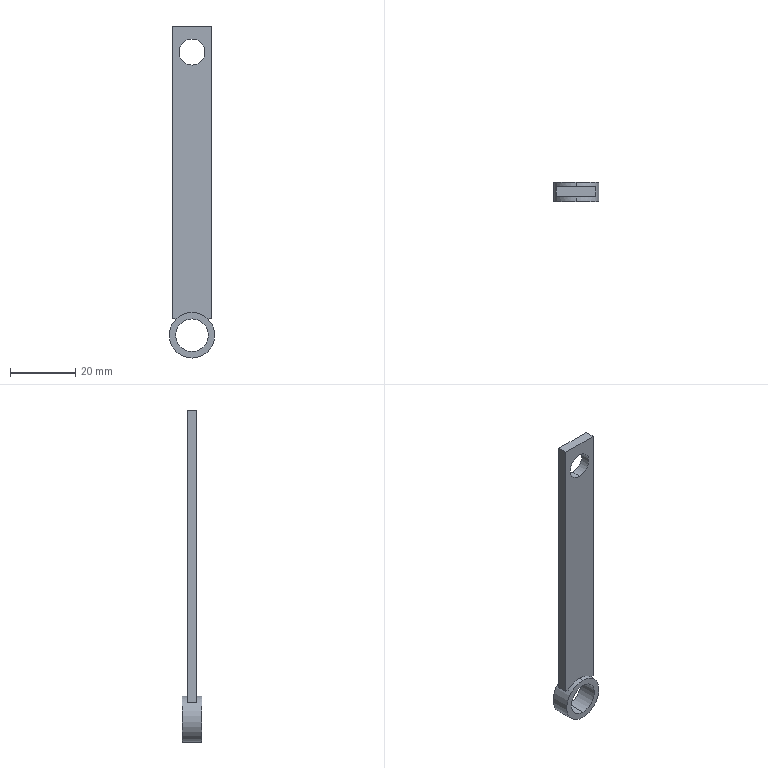Part | NX | features BREP 1 | 1 solid | 15 faces | box 14 x 6 x 102 mm | volume 3501 mm3 | plane 9 | cylinder 6 | commonest cylinder face diameters 8 x2 10 x2 14 x2
STEP:
#1=CARTESIAN_POINT('',(0.,3.,-55.));
#2=VERTEX_POINT('',#1);
#3=CARTESIAN_POINT('',(0.,3.,-45.));
#4=VERTEX_POINT('',#3);
#5=CARTESIAN_POINT('',(0.,3.,-50.));
#6=DIRECTION('',(0.,1.,0.));
#7=DIRECTION('',(0.,0.,1.));
#8=AXIS2_PLACEMENT_3D('',#5,#6,#7);
#9=CIRCLE('',#8,5.);
#10=EDGE_CURVE('',#2,#4,#9,.T.);
#11=ORIENTED_EDGE('',*,*,#10,.T.);
#12=CARTESIAN_POINT('',(0.,-3.,-45.));
#13=VERTEX_POINT('',#12);
#14=CARTESIAN_POINT('',(0.,3.,-45.));
#15=DIRECTION('',(0.,-1.,0.));
#16=VECTOR('',#15,1000.);
#17=LINE('',#14,#16);
#18=EDGE_CURVE('',#13,#4,#17,.F.);
#19=ORIENTED_EDGE('',*,*,#18,.F.);
#20=CARTESIAN_POINT('',(0.,-3.,-55.));
#21=VERTEX_POINT('',#20);
#22=CARTESIAN_POINT('',(0.,-3.,-50.));
#23=DIRECTION('',(0.,1.,0.));
#24=DIRECTION('',(0.,0.,1.));
#25=AXIS2_PLACEMENT_3D('',#22,#23,#24);
#26=CIRCLE('',#25,5.);
#27=EDGE_CURVE('',#21,#13,#26,.T.);
#28=ORIENTED_EDGE('',*,*,#27,.F.);
#29=CARTESIAN_POINT('',(0.,3.,-55.));
#30=DIRECTION('',(0.,-1.,0.));
#31=VECTOR('',#30,1000.);
#32=LINE('',#29,#31);
#33=EDGE_CURVE('',#21,#2,#32,.F.);
#34=ORIENTED_EDGE('',*,*,#33,.T.);
#35=EDGE_LOOP('',(#11,#19,#28,#34));
#36=FACE_BOUND('',#35,.T.);
#37=CARTESIAN_POINT('',(0.,3.,-50.));
#38=DIRECTION('',(0.,-1.,0.));
#39=DIRECTION('',(0.,0.,1.));
#40=AXIS2_PLACEMENT_3D('',#37,#38,#39);
#41=CYLINDRICAL_SURFACE('',#40,5.);
#42=ADVANCED_FACE('',(#36),#41,.F.);
#43=CARTESIAN_POINT('',(0.,3.,-43.));
#44=VERTEX_POINT('',#43);
#45=CARTESIAN_POINT('',(0.,3.,-57.));
#46=VERTEX_POINT('',#45);
#47=CARTESIAN_POINT('',(0.,3.,-50.));
#48=DIRECTION('',(0.,1.,0.));
#49=DIRECTION('',(0.,0.,1.));
#50=AXIS2_PLACEMENT_3D('',#47,#48,#49);
#51=CIRCLE('',#50,7.);
#52=EDGE_CURVE('',#44,#46,#51,.T.);
#53=ORIENTED_EDGE('',*,*,#52,.F.);
#54=CARTESIAN_POINT('',(0.,1.5,-43.));
#55=VERTEX_POINT('',#54);
#56=CARTESIAN_POINT('',(0.,3.,-43.));
#57=DIRECTION('',(0.,-1.,0.));
#58=VECTOR('',#57,1000.);
#59=LINE('',#56,#58);
#60=EDGE_CURVE('',#55,#44,#59,.F.);
#61=ORIENTED_EDGE('',*,*,#60,.F.);
#62=CARTESIAN_POINT('',(4.899,1.5,-45.));
#63=VERTEX_POINT('',#62);
#64=CARTESIAN_POINT('',(0.,1.5,-50.));
#65=DIRECTION('',(0.,1.,0.));
#66=DIRECTION('',(0.,0.,-1.));
#67=AXIS2_PLACEMENT_3D('',#64,#65,#66);
#68=CIRCLE('',#67,7.);
#69=EDGE_CURVE('',#55,#63,#68,.T.);
#70=ORIENTED_EDGE('',*,*,#69,.T.);
#71=CARTESIAN_POINT('',(4.899,-1.5,-45.));
#72=VERTEX_POINT('',#71);
#73=CARTESIAN_POINT('',(4.899,3.,-45.));
#74=DIRECTION('',(0.,-1.,0.));
#75=VECTOR('',#74,1000.);
#76=LINE('',#73,#75);
#77=EDGE_CURVE('',#63,#72,#76,.T.);
#78=ORIENTED_EDGE('',*,*,#77,.T.);
#79=CARTESIAN_POINT('',(0.,-1.5,-43.));
#80=VERTEX_POINT('',#79);
#81=CARTESIAN_POINT('',(0.,-1.5,-50.));
#82=DIRECTION('',(0.,1.,0.));
#83=DIRECTION('',(0.,0.,-1.));
#84=AXIS2_PLACEMENT_3D('',#81,#82,#83);
#85=CIRCLE('',#84,7.);
#86=EDGE_CURVE('',#80,#72,#85,.T.);
#87=ORIENTED_EDGE('',*,*,#86,.F.);
#88=CARTESIAN_POINT('',(0.,-3.,-43.));
#89=VERTEX_POINT('',#88);
#90=CARTESIAN_POINT('',(0.,3.,-43.));
#91=DIRECTION('',(0.,-1.,0.));
#92=VECTOR('',#91,1000.);
#93=LINE('',#90,#92);
#94=EDGE_CURVE('',#80,#89,#93,.T.);
#95=ORIENTED_EDGE('',*,*,#94,.T.);
#96=CARTESIAN_POINT('',(0.,-3.,-57.));
#97=VERTEX_POINT('',#96);
#98=CARTESIAN_POINT('',(0.,-3.,-50.));
#99=DIRECTION('',(0.,1.,0.));
#100=DIRECTION('',(0.,0.,1.));
#101=AXIS2_PLACEMENT_3D('',#98,#99,#100);
#102=CIRCLE('',#101,7.);
#103=EDGE_CURVE('',#89,#97,#102,.T.);
#104=ORIENTED_EDGE('',*,*,#103,.T.);
#105=CARTESIAN_POINT('',(0.,3.,-57.));
#106=DIRECTION('',(0.,-1.,0.));
#107=VECTOR('',#106,1000.);
#108=LINE('',#105,#107);
#109=EDGE_CURVE('',#97,#46,#108,.F.);
#110=ORIENTED_EDGE('',*,*,#109,.T.);
#111=EDGE_LOOP('',(#53,#61,#70,#78,#87,#95,#104,#110));
#112=FACE_BOUND('',#111,.T.);
#113=CARTESIAN_POINT('',(0.,3.,-50.));
#114=DIRECTION('',(0.,-1.,0.));
#115=DIRECTION('',(0.,0.,1.));
#116=AXIS2_PLACEMENT_3D('',#113,#114,#115);
#117=CYLINDRICAL_SURFACE('',#116,7.);
#118=ADVANCED_FACE('',(#112),#117,.T.);
#119=CARTESIAN_POINT('',(0.,1.5,33.));
#120=VERTEX_POINT('',#119);
#121=CARTESIAN_POINT('',(0.,1.5,41.));
#122=VERTEX_POINT('',#121);
#123=CARTESIAN_POINT('',(0.,1.5,37.));
#124=DIRECTION('',(0.,1.,0.));
#125=DIRECTION('',(0.,0.,1.));
#126=AXIS2_PLACEMENT_3D('',#123,#124,#125);
#127=CIRCLE('',#126,4.);
#128=EDGE_CURVE('',#120,#122,#127,.T.);
#129=ORIENTED_EDGE('',*,*,#128,.T.);
#130=CARTESIAN_POINT('',(0.,-1.5,41.));
#131=VERTEX_POINT('',#130);
#132=CARTESIAN_POINT('',(0.,1.5,41.));
#133=DIRECTION('',(0.,-1.,0.));
#134=VECTOR('',#133,1000.);
#135=LINE('',#132,#134);
#136=EDGE_CURVE('',#131,#122,#135,.F.);
#137=ORIENTED_EDGE('',*,*,#136,.F.);
#138=CARTESIAN_POINT('',(0.,-1.5,33.));
#139=VERTEX_POINT('',#138);
#140=CARTESIAN_POINT('',(0.,-1.5,37.));
#141=DIRECTION('',(0.,1.,0.));
#142=DIRECTION('',(0.,0.,1.));
#143=AXIS2_PLACEMENT_3D('',#140,#141,#142);
#144=CIRCLE('',#143,4.);
#145=EDGE_CURVE('',#139,#131,#144,.T.);
#146=ORIENTED_EDGE('',*,*,#145,.F.);
#147=CARTESIAN_POINT('',(0.,1.5,33.));
#148=DIRECTION('',(0.,-1.,0.));
#149=VECTOR('',#148,1000.);
#150=LINE('',#147,#149);
#151=EDGE_CURVE('',#139,#120,#150,.F.);
#152=ORIENTED_EDGE('',*,*,#151,.T.);
#153=EDGE_LOOP('',(#129,#137,#146,#152));
#154=FACE_BOUND('',#153,.T.);
#155=CARTESIAN_POINT('',(0.,1.5,37.));
#156=DIRECTION('',(0.,-1.,0.));
#157=DIRECTION('',(0.,0.,1.));
#158=AXIS2_PLACEMENT_3D('',#155,#156,#157);
#159=CYLINDRICAL_SURFACE('',#158,4.);
#160=ADVANCED_FACE('',(#154),#159,.F.);
#161=CARTESIAN_POINT('',(-4.899,1.5,-45.));
#162=VERTEX_POINT('',#161);
#163=CARTESIAN_POINT('',(0.,1.5,-50.));
#164=DIRECTION('',(0.,1.,0.));
#165=DIRECTION('',(0.,0.,-1.));
#166=AXIS2_PLACEMENT_3D('',#163,#164,#165);
#167=CIRCLE('',#166,7.);
#168=EDGE_CURVE('',#162,#55,#167,.T.);
#169=ORIENTED_EDGE('',*,*,#168,.F.);
#170=CARTESIAN_POINT('',(-6.,1.5,-45.));
#171=VERTEX_POINT('',#170);
#172=CARTESIAN_POINT('',(-6.,1.5,-45.));
#173=DIRECTION('',(-1.,0.,0.));
#174=VECTOR('',#173,1000.);
#175=LINE('',#172,#174);
#176=EDGE_CURVE('',#162,#171,#175,.T.);
#177=ORIENTED_EDGE('',*,*,#176,.T.);
#178=CARTESIAN_POINT('',(-6.,1.5,45.));
#179=VERTEX_POINT('',#178);
#180=CARTESIAN_POINT('',(-6.,1.5,45.));
#181=DIRECTION('',(0.,0.,1.));
#182=VECTOR('',#181,1000.);
#183=LINE('',#180,#182);
#184=EDGE_CURVE('',#171,#179,#183,.T.);
#185=ORIENTED_EDGE('',*,*,#184,.T.);
#186=CARTESIAN_POINT('',(6.,1.5,45.));
#187=VERTEX_POINT('',#186);
#188=CARTESIAN_POINT('',(-6.,1.5,45.));
#189=DIRECTION('',(1.,0.,0.));
#190=VECTOR('',#189,1000.);
#191=LINE('',#188,#190);
#192=EDGE_CURVE('',#179,#187,#191,.T.);
#193=ORIENTED_EDGE('',*,*,#192,.T.);
#194=CARTESIAN_POINT('',(6.,1.5,-45.));
#195=VERTEX_POINT('',#194);
#196=CARTESIAN_POINT('',(6.,1.5,45.));
#197=DIRECTION('',(0.,0.,-1.));
#198=VECTOR('',#197,1000.);
#199=LINE('',#196,#198);
#200=EDGE_CURVE('',#187,#195,#199,.T.);
#201=ORIENTED_EDGE('',*,*,#200,.T.);
#202=CARTESIAN_POINT('',(-6.,1.5,-45.));
#203=DIRECTION('',(-1.,0.,0.));
#204=VECTOR('',#203,1000.);
#205=LINE('',#202,#204);
#206=EDGE_CURVE('',#195,#63,#205,.T.);
#207=ORIENTED_EDGE('',*,*,#206,.T.);
#208=ORIENTED_EDGE('',*,*,#69,.F.);
#209=EDGE_LOOP('',(#169,#177,#185,#193,#201,#207,#208));
#210=FACE_BOUND('',#209,.T.);
#211=ORIENTED_EDGE('',*,*,#128,.F.);
#212=CARTESIAN_POINT('',(0.,1.5,37.));
#213=DIRECTION('',(0.,1.,0.));
#214=DIRECTION('',(0.,0.,1.));
#215=AXIS2_PLACEMENT_3D('',#212,#213,#214);
#216=CIRCLE('',#215,4.);
#217=EDGE_CURVE('',#122,#120,#216,.T.);
#218=ORIENTED_EDGE('',*,*,#217,.F.);
#219=EDGE_LOOP('',(#211,#218));
#220=FACE_BOUND('',#219,.T.);
#221=CARTESIAN_POINT('',(0.,1.5,0.));
#222=DIRECTION('',(0.,-1.,0.));
#223=DIRECTION('',(0.,0.,1.));
#224=AXIS2_PLACEMENT_3D('',#221,#222,#223);
#225=PLANE('',#224);
#226=ADVANCED_FACE('',(#210,#220),#225,.F.);
#227=CARTESIAN_POINT('',(-4.899,-1.5,-45.));
#228=VERTEX_POINT('',#227);
#229=CARTESIAN_POINT('',(-6.,-1.5,-45.));
#230=VERTEX_POINT('',#229);
#231=CARTESIAN_POINT('',(-6.,-1.5,-45.));
#232=DIRECTION('',(-1.,0.,0.));
#233=VECTOR('',#232,1000.);
#234=LINE('',#231,#233);
#235=EDGE_CURVE('',#228,#230,#234,.T.);
#236=ORIENTED_EDGE('',*,*,#235,.F.);
#237=CARTESIAN_POINT('',(0.,-1.5,-50.));
#238=DIRECTION('',(0.,1.,0.));
#239=DIRECTION('',(0.,0.,-1.));
#240=AXIS2_PLACEMENT_3D('',#237,#238,#239);
#241=CIRCLE('',#240,7.);
#242=EDGE_CURVE('',#228,#80,#241,.T.);
#243=ORIENTED_EDGE('',*,*,#242,.T.);
#244=ORIENTED_EDGE('',*,*,#86,.T.);
#245=CARTESIAN_POINT('',(6.,-1.5,-45.));
#246=VERTEX_POINT('',#245);
#247=CARTESIAN_POINT('',(-6.,-1.5,-45.));
#248=DIRECTION('',(-1.,0.,0.));
#249=VECTOR('',#248,1000.);
#250=LINE('',#247,#249);
#251=EDGE_CURVE('',#246,#72,#250,.T.);
#252=ORIENTED_EDGE('',*,*,#251,.F.);
#253=CARTESIAN_POINT('',(6.,-1.5,45.));
#254=VERTEX_POINT('',#253);
#255=CARTESIAN_POINT('',(6.,-1.5,45.));
#256=DIRECTION('',(0.,0.,-1.));
#257=VECTOR('',#256,1000.);
#258=LINE('',#255,#257);
#259=EDGE_CURVE('',#254,#246,#258,.T.);
#260=ORIENTED_EDGE('',*,*,#259,.F.);
#261=CARTESIAN_POINT('',(-6.,-1.5,45.));
#262=VERTEX_POINT('',#261);
#263=CARTESIAN_POINT('',(-6.,-1.5,45.));
#264=DIRECTION('',(1.,0.,0.));
#265=VECTOR('',#264,1000.);
#266=LINE('',#263,#265);
#267=EDGE_CURVE('',#262,#254,#266,.T.);
#268=ORIENTED_EDGE('',*,*,#267,.F.);
#269=CARTESIAN_POINT('',(-6.,-1.5,45.));
#270=DIRECTION('',(0.,0.,1.));
#271=VECTOR('',#270,1000.);
#272=LINE('',#269,#271);
#273=EDGE_CURVE('',#230,#262,#272,.T.);
#274=ORIENTED_EDGE('',*,*,#273,.F.);
#275=EDGE_LOOP('',(#236,#243,#244,#252,#260,#268,#274));
#276=FACE_BOUND('',#275,.T.);
#277=ORIENTED_EDGE('',*,*,#145,.T.);
#278=CARTESIAN_POINT('',(0.,-1.5,37.));
#279=DIRECTION('',(0.,1.,0.));
#280=DIRECTION('',(0.,0.,1.));
#281=AXIS2_PLACEMENT_3D('',#278,#279,#280);
#282=CIRCLE('',#281,4.);
#283=EDGE_CURVE('',#131,#139,#282,.T.);
#284=ORIENTED_EDGE('',*,*,#283,.T.);
#285=EDGE_LOOP('',(#277,#284));
#286=FACE_BOUND('',#285,.T.);
#287=CARTESIAN_POINT('',(0.,-1.5,0.));
#288=DIRECTION('',(0.,-1.,0.));
#289=DIRECTION('',(0.,0.,1.));
#290=AXIS2_PLACEMENT_3D('',#287,#288,#289);
#291=PLANE('',#290);
#292=ADVANCED_FACE('',(#276,#286),#291,.T.);
#293=CARTESIAN_POINT('',(-4.899,3.,-45.));
#294=DIRECTION('',(0.,1.,0.));
#295=VECTOR('',#294,1000.);
#296=LINE('',#293,#295);
#297=EDGE_CURVE('',#228,#162,#296,.T.);
#298=ORIENTED_EDGE('',*,*,#297,.F.);
#299=ORIENTED_EDGE('',*,*,#235,.T.);
#300=CARTESIAN_POINT('',(-6.,1.5,-45.));
#301=DIRECTION('',(0.,-1.,0.));
#302=VECTOR('',#301,1000.);
#303=LINE('',#300,#302);
#304=EDGE_CURVE('',#171,#230,#303,.T.);
#305=ORIENTED_EDGE('',*,*,#304,.F.);
#306=ORIENTED_EDGE('',*,*,#176,.F.);
#307=EDGE_LOOP('',(#298,#299,#305,#306));
#308=FACE_BOUND('',#307,.T.);
#309=CARTESIAN_POINT('',(-6.,1.5,-45.));
#310=DIRECTION('',(0.,0.,1.));
#311=DIRECTION('',(-1.,0.,0.));
#312=AXIS2_PLACEMENT_3D('',#309,#310,#311);
#313=PLANE('',#312);
#314=ADVANCED_FACE('',(#308),#313,.F.);
#315=ORIENTED_EDGE('',*,*,#77,.F.);
#316=ORIENTED_EDGE('',*,*,#206,.F.);
#317=CARTESIAN_POINT('',(6.,1.5,-45.));
#318=DIRECTION('',(0.,-1.,0.));
#319=VECTOR('',#318,1000.);
#320=LINE('',#317,#319);
#321=EDGE_CURVE('',#195,#246,#320,.T.);
#322=ORIENTED_EDGE('',*,*,#321,.T.);
#323=ORIENTED_EDGE('',*,*,#251,.T.);
#324=EDGE_LOOP('',(#315,#316,#322,#323));
#325=FACE_BOUND('',#324,.T.);
#326=CARTESIAN_POINT('',(-6.,1.5,-45.));
#327=DIRECTION('',(0.,0.,1.));
#328=DIRECTION('',(-1.,0.,0.));
#329=AXIS2_PLACEMENT_3D('',#326,#327,#328);
#330=PLANE('',#329);
#331=ADVANCED_FACE('',(#325),#330,.F.);
#332=ORIENTED_EDGE('',*,*,#259,.T.);
#333=ORIENTED_EDGE('',*,*,#321,.F.);
#334=ORIENTED_EDGE('',*,*,#200,.F.);
#335=CARTESIAN_POINT('',(6.,1.5,45.));
#336=DIRECTION('',(0.,-1.,0.));
#337=VECTOR('',#336,1000.);
#338=LINE('',#335,#337);
#339=EDGE_CURVE('',#187,#254,#338,.T.);
#340=ORIENTED_EDGE('',*,*,#339,.T.);
#341=EDGE_LOOP('',(#332,#333,#334,#340));
#342=FACE_BOUND('',#341,.T.);
#343=CARTESIAN_POINT('',(6.,1.5,45.));
#344=DIRECTION('',(-1.,0.,0.));
#345=DIRECTION('',(0.,0.,-1.));
#346=AXIS2_PLACEMENT_3D('',#343,#344,#345);
#347=PLANE('',#346);
#348=ADVANCED_FACE('',(#342),#347,.F.);
#349=ORIENTED_EDGE('',*,*,#273,.T.);
#350=CARTESIAN_POINT('',(-6.,1.5,45.));
#351=DIRECTION('',(0.,-1.,0.));
#352=VECTOR('',#351,1000.);
#353=LINE('',#350,#352);
#354=EDGE_CURVE('',#179,#262,#353,.T.);
#355=ORIENTED_EDGE('',*,*,#354,.F.);
#356=ORIENTED_EDGE('',*,*,#184,.F.);
#357=ORIENTED_EDGE('',*,*,#304,.T.);
#358=EDGE_LOOP('',(#349,#355,#356,#357));
#359=FACE_BOUND('',#358,.T.);
#360=CARTESIAN_POINT('',(-6.,1.5,45.));
#361=DIRECTION('',(1.,0.,0.));
#362=DIRECTION('',(0.,-1.,0.));
#363=AXIS2_PLACEMENT_3D('',#360,#361,#362);
#364=PLANE('',#363);
#365=ADVANCED_FACE('',(#359),#364,.F.);
#366=ORIENTED_EDGE('',*,*,#267,.T.);
#367=ORIENTED_EDGE('',*,*,#339,.F.);
#368=ORIENTED_EDGE('',*,*,#192,.F.);
#369=ORIENTED_EDGE('',*,*,#354,.T.);
#370=EDGE_LOOP('',(#366,#367,#368,#369));
#371=FACE_BOUND('',#370,.T.);
#372=CARTESIAN_POINT('',(-6.,1.5,45.));
#373=DIRECTION('',(0.,0.,-1.));
#374=DIRECTION('',(0.,1.,0.));
#375=AXIS2_PLACEMENT_3D('',#372,#373,#374);
#376=PLANE('',#375);
#377=ADVANCED_FACE('',(#371),#376,.F.);
#378=ORIENTED_EDGE('',*,*,#136,.T.);
#379=ORIENTED_EDGE('',*,*,#217,.T.);
#380=ORIENTED_EDGE('',*,*,#151,.F.);
#381=ORIENTED_EDGE('',*,*,#283,.F.);
#382=EDGE_LOOP('',(#378,#379,#380,#381));
#383=FACE_BOUND('',#382,.T.);
#384=CARTESIAN_POINT('',(0.,1.5,37.));
#385=DIRECTION('',(0.,-1.,0.));
#386=DIRECTION('',(0.,0.,1.));
#387=AXIS2_PLACEMENT_3D('',#384,#385,#386);
#388=CYLINDRICAL_SURFACE('',#387,4.);
#389=ADVANCED_FACE('',(#383),#388,.F.);
#390=ORIENTED_EDGE('',*,*,#60,.T.);
#391=CARTESIAN_POINT('',(0.,3.,-50.));
#392=DIRECTION('',(0.,1.,0.));
#393=DIRECTION('',(0.,0.,1.));
#394=AXIS2_PLACEMENT_3D('',#391,#392,#393);
#395=CIRCLE('',#394,7.);
#396=EDGE_CURVE('',#46,#44,#395,.T.);
#397=ORIENTED_EDGE('',*,*,#396,.F.);
#398=ORIENTED_EDGE('',*,*,#109,.F.);
#399=CARTESIAN_POINT('',(0.,-3.,-50.));
#400=DIRECTION('',(0.,1.,0.));
#401=DIRECTION('',(0.,0.,1.));
#402=AXIS2_PLACEMENT_3D('',#399,#400,#401);
#403=CIRCLE('',#402,7.);
#404=EDGE_CURVE('',#97,#89,#403,.T.);
#405=ORIENTED_EDGE('',*,*,#404,.T.);
#406=ORIENTED_EDGE('',*,*,#94,.F.);
#407=ORIENTED_EDGE('',*,*,#242,.F.);
#408=ORIENTED_EDGE('',*,*,#297,.T.);
#409=ORIENTED_EDGE('',*,*,#168,.T.);
#410=EDGE_LOOP('',(#390,#397,#398,#405,#406,#407,#408,#409));
#411=FACE_BOUND('',#410,.T.);
#412=CARTESIAN_POINT('',(0.,3.,-50.));
#413=DIRECTION('',(0.,-1.,0.));
#414=DIRECTION('',(0.,0.,1.));
#415=AXIS2_PLACEMENT_3D('',#412,#413,#414);
#416=CYLINDRICAL_SURFACE('',#415,7.);
#417=ADVANCED_FACE('',(#411),#416,.T.);
#418=ORIENTED_EDGE('',*,*,#396,.T.);
#419=ORIENTED_EDGE('',*,*,#52,.T.);
#420=EDGE_LOOP('',(#418,#419));
#421=FACE_BOUND('',#420,.T.);
#422=ORIENTED_EDGE('',*,*,#10,.F.);
#423=CARTESIAN_POINT('',(0.,3.,-50.));
#424=DIRECTION('',(0.,1.,0.));
#425=DIRECTION('',(0.,0.,1.));
#426=AXIS2_PLACEMENT_3D('',#423,#424,#425);
#427=CIRCLE('',#426,5.);
#428=EDGE_CURVE('',#4,#2,#427,.T.);
#429=ORIENTED_EDGE('',*,*,#428,.F.);
#430=EDGE_LOOP('',(#422,#429));
#431=FACE_BOUND('',#430,.T.);
#432=CARTESIAN_POINT('',(0.,3.,-50.));
#433=DIRECTION('',(0.,1.,0.));
#434=DIRECTION('',(-1.,0.,0.));
#435=AXIS2_PLACEMENT_3D('',#432,#433,#434);
#436=PLANE('',#435);
#437=ADVANCED_FACE('',(#421,#431),#436,.T.);
#438=ORIENTED_EDGE('',*,*,#404,.F.);
#439=ORIENTED_EDGE('',*,*,#103,.F.);
#440=EDGE_LOOP('',(#438,#439));
#441=FACE_BOUND('',#440,.T.);
#442=ORIENTED_EDGE('',*,*,#27,.T.);
#443=CARTESIAN_POINT('',(0.,-3.,-50.));
#444=DIRECTION('',(0.,1.,0.));
#445=DIRECTION('',(0.,0.,1.));
#446=AXIS2_PLACEMENT_3D('',#443,#444,#445);
#447=CIRCLE('',#446,5.);
#448=EDGE_CURVE('',#13,#21,#447,.T.);
#449=ORIENTED_EDGE('',*,*,#448,.T.);
#450=EDGE_LOOP('',(#442,#449));
#451=FACE_BOUND('',#450,.T.);
#452=CARTESIAN_POINT('',(0.,-3.,-50.));
#453=DIRECTION('',(0.,1.,0.));
#454=DIRECTION('',(-1.,0.,0.));
#455=AXIS2_PLACEMENT_3D('',#452,#453,#454);
#456=PLANE('',#455);
#457=ADVANCED_FACE('',(#441,#451),#456,.F.);
#458=ORIENTED_EDGE('',*,*,#18,.T.);
#459=ORIENTED_EDGE('',*,*,#428,.T.);
#460=ORIENTED_EDGE('',*,*,#33,.F.);
#461=ORIENTED_EDGE('',*,*,#448,.F.);
#462=EDGE_LOOP('',(#458,#459,#460,#461));
#463=FACE_BOUND('',#462,.T.);
#464=CARTESIAN_POINT('',(0.,3.,-50.));
#465=DIRECTION('',(0.,-1.,0.));
#466=DIRECTION('',(0.,0.,1.));
#467=AXIS2_PLACEMENT_3D('',#464,#465,#466);
#468=CYLINDRICAL_SURFACE('',#467,5.);
#469=ADVANCED_FACE('',(#463),#468,.F.);
#470=CLOSED_SHELL('',(#42,#118,#160,#226,#292,#314,#331,#348,#365,#377,#389,#417,#437,#457,#469));
#471=MANIFOLD_SOLID_BREP('',#470);
#472=(LENGTH_UNIT()NAMED_UNIT(*)SI_UNIT(.MILLI.,.METRE.));
#473=UNCERTAINTY_MEASURE_WITH_UNIT(LENGTH_MEASURE(0.00001),#472,'','');
#474=(NAMED_UNIT(*)PLANE_ANGLE_UNIT()SI_UNIT($,.RADIAN.));
#475=(NAMED_UNIT(*)SI_UNIT($,.STERADIAN.)SOLID_ANGLE_UNIT());
#476=(GEOMETRIC_REPRESENTATION_CONTEXT(3)GLOBAL_UNCERTAINTY_ASSIGNED_CONTEXT((#473))GLOBAL_UNIT_ASSIGNED_CONTEXT((#472,#474,#475))REPRESENTATION_CONTEXT('',''));
#477=ADVANCED_BREP_SHAPE_REPRESENTATION('',(#471),#476);